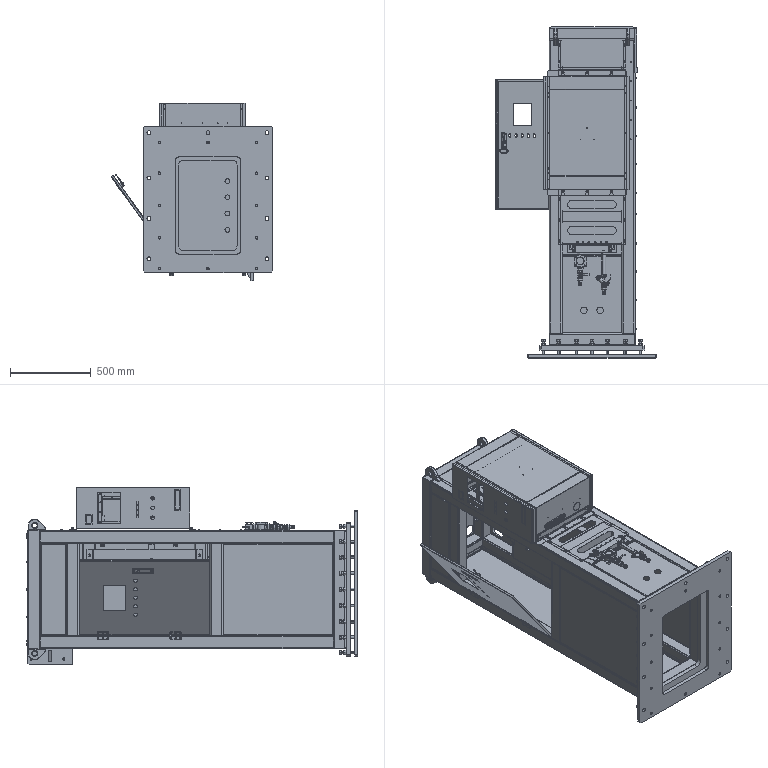Part | SolidWorks | features ReferencePattern 14, LocalLPattern 1 | 566 solids | 12594 faces | volume 53716984 mm3 | cylinder 5406 | plane 5213 | cone 1162 | torus 674 | spline 131 | sphere 8 | commonest cylinder face diameters 4.5 x583 4 x527 5 x465 3.3 x376 4.1 x339 6.287 x339